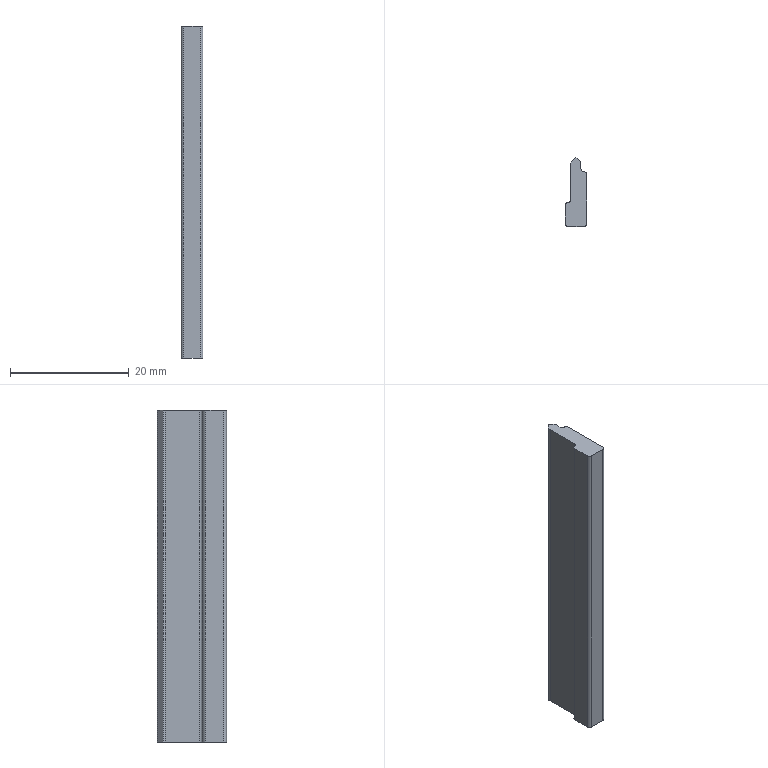Part | NX | features BREP 2 | 2 solids | 34 faces | box 3.7 x 11.653 x 56 mm | volume 3605 mm3 | plane 18 | cylinder 16 | commonest cylinder face diameters 1 x16
STEP:
#1=CARTESIAN_POINT('',(0.6935,5.13,-4.));
#2=VERTEX_POINT('',#1);
#3=CARTESIAN_POINT('',(0.6935,5.13,52.));
#4=VERTEX_POINT('',#3);
#5=CARTESIAN_POINT('',(0.6935,5.13,0.));
#6=DIRECTION('',(0.,0.,1.));
#7=VECTOR('',#6,1000.);
#8=LINE('',#5,#7);
#9=EDGE_CURVE('',#2,#4,#8,.T.);
#10=ORIENTED_EDGE('',*,*,#9,.T.);
#11=CARTESIAN_POINT('',(0.8399,4.776,52.));
#12=VERTEX_POINT('',#11);
#13=CARTESIAN_POINT('',(0.3399,4.776,52.));
#14=DIRECTION('',(0.,0.,1.));
#15=DIRECTION('',(1.,0.,0.));
#16=AXIS2_PLACEMENT_3D('',#13,#14,#15);
#17=CIRCLE('',#16,0.5);
#18=EDGE_CURVE('',#12,#4,#17,.T.);
#19=ORIENTED_EDGE('',*,*,#18,.F.);
#20=CARTESIAN_POINT('',(0.8399,4.776,-4.));
#21=VERTEX_POINT('',#20);
#22=CARTESIAN_POINT('',(0.8399,4.776,0.));
#23=DIRECTION('',(0.,0.,1.));
#24=VECTOR('',#23,1000.);
#25=LINE('',#22,#24);
#26=EDGE_CURVE('',#21,#12,#25,.T.);
#27=ORIENTED_EDGE('',*,*,#26,.F.);
#28=CARTESIAN_POINT('',(0.3399,4.776,-4.));
#29=DIRECTION('',(0.,0.,1.));
#30=DIRECTION('',(1.,0.,0.));
#31=AXIS2_PLACEMENT_3D('',#28,#29,#30);
#32=CIRCLE('',#31,0.5);
#33=EDGE_CURVE('',#21,#2,#32,.T.);
#34=ORIENTED_EDGE('',*,*,#33,.T.);
#35=EDGE_LOOP('',(#10,#19,#27,#34));
#36=FACE_BOUND('',#35,.T.);
#37=CARTESIAN_POINT('',(0.3399,4.776,0.));
#38=DIRECTION('',(0.,0.,1.));
#39=DIRECTION('',(-1.,0.,0.));
#40=AXIS2_PLACEMENT_3D('',#37,#38,#39);
#41=CYLINDRICAL_SURFACE('',#40,0.5);
#42=ADVANCED_FACE('',(#36),#41,.T.);
#43=ORIENTED_EDGE('',*,*,#26,.T.);
#44=CARTESIAN_POINT('',(0.8399,3.873,52.));
#45=VERTEX_POINT('',#44);
#46=CARTESIAN_POINT('',(0.8399,-7.849,52.));
#47=DIRECTION('',(0.,1.,0.));
#48=VECTOR('',#47,1000.);
#49=LINE('',#46,#48);
#50=EDGE_CURVE('',#45,#12,#49,.T.);
#51=ORIENTED_EDGE('',*,*,#50,.F.);
#52=CARTESIAN_POINT('',(0.8399,3.873,-4.));
#53=VERTEX_POINT('',#52);
#54=CARTESIAN_POINT('',(0.8399,3.873,0.));
#55=DIRECTION('',(0.,0.,1.));
#56=VECTOR('',#55,1000.);
#57=LINE('',#54,#56);
#58=EDGE_CURVE('',#53,#45,#57,.T.);
#59=ORIENTED_EDGE('',*,*,#58,.F.);
#60=CARTESIAN_POINT('',(0.8399,-7.849,-4.));
#61=DIRECTION('',(0.,1.,0.));
#62=VECTOR('',#61,1000.);
#63=LINE('',#60,#62);
#64=EDGE_CURVE('',#53,#21,#63,.T.);
#65=ORIENTED_EDGE('',*,*,#64,.T.);
#66=EDGE_LOOP('',(#43,#51,#59,#65));
#67=FACE_BOUND('',#66,.T.);
#68=CARTESIAN_POINT('',(0.8399,4.776,0.));
#69=DIRECTION('',(-1.,0.,0.));
#70=DIRECTION('',(0.,1.,0.));
#71=AXIS2_PLACEMENT_3D('',#68,#69,#70);
#72=PLANE('',#71);
#73=ADVANCED_FACE('',(#67),#72,.F.);
#74=ORIENTED_EDGE('',*,*,#58,.T.);
#75=CARTESIAN_POINT('',(1.35,3.373,52.));
#76=VERTEX_POINT('',#75);
#77=CARTESIAN_POINT('',(1.34,3.873,52.));
#78=DIRECTION('',(0.,0.,-1.));
#79=DIRECTION('',(1.,0.,0.));
#80=AXIS2_PLACEMENT_3D('',#77,#78,#79);
#81=CIRCLE('',#80,0.5);
#82=EDGE_CURVE('',#76,#45,#81,.T.);
#83=ORIENTED_EDGE('',*,*,#82,.F.);
#84=CARTESIAN_POINT('',(1.35,3.373,-4.));
#85=VERTEX_POINT('',#84);
#86=CARTESIAN_POINT('',(1.35,3.373,52.));
#87=CARTESIAN_POINT('',(1.35,3.373,33.333));
#88=CARTESIAN_POINT('',(1.35,3.373,14.667));
#89=CARTESIAN_POINT('',(1.35,3.373,-4.));
#90=B_SPLINE_CURVE_WITH_KNOTS('',3,(#86,#87,#88,#89),.UNSPECIFIED.,.F.,.F.,(4,4),(0.,1.),.UNSPECIFIED.);
#91=EDGE_CURVE('',#85,#76,#90,.F.);
#92=ORIENTED_EDGE('',*,*,#91,.F.);
#93=CARTESIAN_POINT('',(1.34,3.873,-4.));
#94=DIRECTION('',(0.,0.,-1.));
#95=DIRECTION('',(1.,0.,0.));
#96=AXIS2_PLACEMENT_3D('',#93,#94,#95);
#97=CIRCLE('',#96,0.5);
#98=EDGE_CURVE('',#85,#53,#97,.T.);
#99=ORIENTED_EDGE('',*,*,#98,.T.);
#100=EDGE_LOOP('',(#74,#83,#92,#99));
#101=FACE_BOUND('',#100,.T.);
#102=CARTESIAN_POINT('',(1.34,3.873,0.));
#103=DIRECTION('',(0.,0.,1.));
#104=DIRECTION('',(-1.,0.,0.));
#105=AXIS2_PLACEMENT_3D('',#102,#103,#104);
#106=CYLINDRICAL_SURFACE('',#105,0.5);
#107=ADVANCED_FACE('',(#101),#106,.F.);
#108=ORIENTED_EDGE('',*,*,#91,.T.);
#109=CARTESIAN_POINT('',(1.85,2.873,52.));
#110=VERTEX_POINT('',#109);
#111=CARTESIAN_POINT('',(1.35,2.873,52.));
#112=DIRECTION('',(0.,0.,1.));
#113=DIRECTION('',(1.,0.,0.));
#114=AXIS2_PLACEMENT_3D('',#111,#112,#113);
#115=CIRCLE('',#114,0.5);
#116=EDGE_CURVE('',#110,#76,#115,.T.);
#117=ORIENTED_EDGE('',*,*,#116,.F.);
#118=CARTESIAN_POINT('',(1.85,2.873,-4.));
#119=VERTEX_POINT('',#118);
#120=CARTESIAN_POINT('',(1.85,2.873,0.));
#121=DIRECTION('',(0.,0.,1.));
#122=VECTOR('',#121,1000.);
#123=LINE('',#120,#122);
#124=EDGE_CURVE('',#119,#110,#123,.T.);
#125=ORIENTED_EDGE('',*,*,#124,.F.);
#126=CARTESIAN_POINT('',(1.35,2.873,-4.));
#127=DIRECTION('',(0.,0.,1.));
#128=DIRECTION('',(1.,0.,0.));
#129=AXIS2_PLACEMENT_3D('',#126,#127,#128);
#130=CIRCLE('',#129,0.5);
#131=EDGE_CURVE('',#119,#85,#130,.T.);
#132=ORIENTED_EDGE('',*,*,#131,.T.);
#133=EDGE_LOOP('',(#108,#117,#125,#132));
#134=FACE_BOUND('',#133,.T.);
#135=CARTESIAN_POINT('',(1.35,2.873,0.));
#136=DIRECTION('',(0.,0.,1.));
#137=DIRECTION('',(-1.,0.,0.));
#138=AXIS2_PLACEMENT_3D('',#135,#136,#137);
#139=CYLINDRICAL_SURFACE('',#138,0.5);
#140=ADVANCED_FACE('',(#134),#139,.T.);
#141=ORIENTED_EDGE('',*,*,#124,.T.);
#142=CARTESIAN_POINT('',(1.85,-5.327,52.));
#143=VERTEX_POINT('',#142);
#144=CARTESIAN_POINT('',(1.85,-7.849,52.));
#145=DIRECTION('',(0.,1.,0.));
#146=VECTOR('',#145,1000.);
#147=LINE('',#144,#146);
#148=EDGE_CURVE('',#143,#110,#147,.T.);
#149=ORIENTED_EDGE('',*,*,#148,.F.);
#150=CARTESIAN_POINT('',(1.85,-5.327,-4.));
#151=VERTEX_POINT('',#150);
#152=CARTESIAN_POINT('',(1.85,-5.327,0.));
#153=DIRECTION('',(0.,0.,1.));
#154=VECTOR('',#153,1000.);
#155=LINE('',#152,#154);
#156=EDGE_CURVE('',#151,#143,#155,.T.);
#157=ORIENTED_EDGE('',*,*,#156,.F.);
#158=CARTESIAN_POINT('',(1.85,-7.849,-4.));
#159=DIRECTION('',(0.,1.,0.));
#160=VECTOR('',#159,1000.);
#161=LINE('',#158,#160);
#162=EDGE_CURVE('',#151,#119,#161,.T.);
#163=ORIENTED_EDGE('',*,*,#162,.T.);
#164=EDGE_LOOP('',(#141,#149,#157,#163));
#165=FACE_BOUND('',#164,.T.);
#166=CARTESIAN_POINT('',(1.85,2.873,0.));
#167=DIRECTION('',(-1.,0.,0.));
#168=DIRECTION('',(0.,1.,0.));
#169=AXIS2_PLACEMENT_3D('',#166,#167,#168);
#170=PLANE('',#169);
#171=ADVANCED_FACE('',(#165),#170,.F.);
#172=ORIENTED_EDGE('',*,*,#156,.T.);
#173=CARTESIAN_POINT('',(1.35,-5.827,52.));
#174=VERTEX_POINT('',#173);
#175=CARTESIAN_POINT('',(1.35,-5.327,52.));
#176=DIRECTION('',(0.,0.,1.));
#177=DIRECTION('',(1.,0.,0.));
#178=AXIS2_PLACEMENT_3D('',#175,#176,#177);
#179=CIRCLE('',#178,0.5);
#180=EDGE_CURVE('',#174,#143,#179,.T.);
#181=ORIENTED_EDGE('',*,*,#180,.F.);
#182=CARTESIAN_POINT('',(1.35,-5.827,-4.));
#183=VERTEX_POINT('',#182);
#184=CARTESIAN_POINT('',(1.35,-5.827,0.));
#185=DIRECTION('',(0.,0.,1.));
#186=VECTOR('',#185,1000.);
#187=LINE('',#184,#186);
#188=EDGE_CURVE('',#183,#174,#187,.T.);
#189=ORIENTED_EDGE('',*,*,#188,.F.);
#190=CARTESIAN_POINT('',(1.35,-5.327,-4.));
#191=DIRECTION('',(0.,0.,1.));
#192=DIRECTION('',(1.,0.,0.));
#193=AXIS2_PLACEMENT_3D('',#190,#191,#192);
#194=CIRCLE('',#193,0.5);
#195=EDGE_CURVE('',#183,#151,#194,.T.);
#196=ORIENTED_EDGE('',*,*,#195,.T.);
#197=EDGE_LOOP('',(#172,#181,#189,#196));
#198=FACE_BOUND('',#197,.T.);
#199=CARTESIAN_POINT('',(1.35,-5.327,0.));
#200=DIRECTION('',(0.,0.,1.));
#201=DIRECTION('',(-1.,0.,0.));
#202=AXIS2_PLACEMENT_3D('',#199,#200,#201);
#203=CYLINDRICAL_SURFACE('',#202,0.5);
#204=ADVANCED_FACE('',(#198),#203,.T.);
#205=ORIENTED_EDGE('',*,*,#188,.T.);
#206=CARTESIAN_POINT('',(-1.35,-5.827,52.));
#207=VERTEX_POINT('',#206);
#208=CARTESIAN_POINT('',(12.323,-5.827,52.));
#209=DIRECTION('',(1.,0.,0.));
#210=VECTOR('',#209,1000.);
#211=LINE('',#208,#210);
#212=EDGE_CURVE('',#207,#174,#211,.T.);
#213=ORIENTED_EDGE('',*,*,#212,.F.);
#214=CARTESIAN_POINT('',(-1.35,-5.827,-4.));
#215=VERTEX_POINT('',#214);
#216=CARTESIAN_POINT('',(-1.35,-5.827,0.));
#217=DIRECTION('',(0.,0.,1.));
#218=VECTOR('',#217,1000.);
#219=LINE('',#216,#218);
#220=EDGE_CURVE('',#215,#207,#219,.T.);
#221=ORIENTED_EDGE('',*,*,#220,.F.);
#222=CARTESIAN_POINT('',(12.323,-5.827,-4.));
#223=DIRECTION('',(1.,0.,0.));
#224=VECTOR('',#223,1000.);
#225=LINE('',#222,#224);
#226=EDGE_CURVE('',#215,#183,#225,.T.);
#227=ORIENTED_EDGE('',*,*,#226,.T.);
#228=EDGE_LOOP('',(#205,#213,#221,#227));
#229=FACE_BOUND('',#228,.T.);
#230=CARTESIAN_POINT('',(1.35,-5.827,0.));
#231=DIRECTION('',(0.,1.,0.));
#232=DIRECTION('',(1.,0.,0.));
#233=AXIS2_PLACEMENT_3D('',#230,#231,#232);
#234=PLANE('',#233);
#235=ADVANCED_FACE('',(#229),#234,.F.);
#236=ORIENTED_EDGE('',*,*,#220,.T.);
#237=CARTESIAN_POINT('',(-1.85,-5.327,52.));
#238=VERTEX_POINT('',#237);
#239=CARTESIAN_POINT('',(-1.35,-5.327,52.));
#240=DIRECTION('',(0.,0.,1.));
#241=DIRECTION('',(1.,0.,0.));
#242=AXIS2_PLACEMENT_3D('',#239,#240,#241);
#243=CIRCLE('',#242,0.5);
#244=EDGE_CURVE('',#238,#207,#243,.T.);
#245=ORIENTED_EDGE('',*,*,#244,.F.);
#246=CARTESIAN_POINT('',(-1.85,-5.327,-4.));
#247=VERTEX_POINT('',#246);
#248=CARTESIAN_POINT('',(-1.85,-5.327,0.));
#249=DIRECTION('',(0.,0.,1.));
#250=VECTOR('',#249,1000.);
#251=LINE('',#248,#250);
#252=EDGE_CURVE('',#247,#238,#251,.T.);
#253=ORIENTED_EDGE('',*,*,#252,.F.);
#254=CARTESIAN_POINT('',(-1.35,-5.327,-4.));
#255=DIRECTION('',(0.,0.,1.));
#256=DIRECTION('',(1.,0.,0.));
#257=AXIS2_PLACEMENT_3D('',#254,#255,#256);
#258=CIRCLE('',#257,0.5);
#259=EDGE_CURVE('',#247,#215,#258,.T.);
#260=ORIENTED_EDGE('',*,*,#259,.T.);
#261=EDGE_LOOP('',(#236,#245,#253,#260));
#262=FACE_BOUND('',#261,.T.);
#263=CARTESIAN_POINT('',(-1.35,-5.327,0.));
#264=DIRECTION('',(0.,0.,1.));
#265=DIRECTION('',(-1.,0.,0.));
#266=AXIS2_PLACEMENT_3D('',#263,#264,#265);
#267=CYLINDRICAL_SURFACE('',#266,0.5);
#268=ADVANCED_FACE('',(#262),#267,.T.);
#269=ORIENTED_EDGE('',*,*,#252,.T.);
#270=CARTESIAN_POINT('',(-1.85,-2.327,52.));
#271=VERTEX_POINT('',#270);
#272=CARTESIAN_POINT('',(-1.85,-7.849,52.));
#273=DIRECTION('',(0.,-1.,0.));
#274=VECTOR('',#273,1000.);
#275=LINE('',#272,#274);
#276=EDGE_CURVE('',#271,#238,#275,.T.);
#277=ORIENTED_EDGE('',*,*,#276,.F.);
#278=CARTESIAN_POINT('',(-1.85,-2.327,-4.));
#279=VERTEX_POINT('',#278);
#280=CARTESIAN_POINT('',(-1.85,-2.327,0.));
#281=DIRECTION('',(0.,0.,1.));
#282=VECTOR('',#281,1000.);
#283=LINE('',#280,#282);
#284=EDGE_CURVE('',#279,#271,#283,.T.);
#285=ORIENTED_EDGE('',*,*,#284,.F.);
#286=CARTESIAN_POINT('',(-1.85,-7.849,-4.));
#287=DIRECTION('',(0.,-1.,0.));
#288=VECTOR('',#287,1000.);
#289=LINE('',#286,#288);
#290=EDGE_CURVE('',#279,#247,#289,.T.);
#291=ORIENTED_EDGE('',*,*,#290,.T.);
#292=EDGE_LOOP('',(#269,#277,#285,#291));
#293=FACE_BOUND('',#292,.T.);
#294=CARTESIAN_POINT('',(-1.85,-5.327,0.));
#295=DIRECTION('',(1.,0.,0.));
#296=DIRECTION('',(0.,-1.,0.));
#297=AXIS2_PLACEMENT_3D('',#294,#295,#296);
#298=PLANE('',#297);
#299=ADVANCED_FACE('',(#293),#298,.F.);
#300=ORIENTED_EDGE('',*,*,#284,.T.);
#301=CARTESIAN_POINT('',(-1.35,-1.827,52.));
#302=VERTEX_POINT('',#301);
#303=CARTESIAN_POINT('',(-1.35,-2.327,52.));
#304=DIRECTION('',(0.,0.,1.));
#305=DIRECTION('',(1.,0.,0.));
#306=AXIS2_PLACEMENT_3D('',#303,#304,#305);
#307=CIRCLE('',#306,0.5);
#308=EDGE_CURVE('',#302,#271,#307,.T.);
#309=ORIENTED_EDGE('',*,*,#308,.F.);
#310=CARTESIAN_POINT('',(-1.35,-1.827,-4.));
#311=VERTEX_POINT('',#310);
#312=CARTESIAN_POINT('',(-1.35,-1.827,0.));
#313=DIRECTION('',(0.,0.,1.));
#314=VECTOR('',#313,1000.);
#315=LINE('',#312,#314);
#316=EDGE_CURVE('',#311,#302,#315,.T.);
#317=ORIENTED_EDGE('',*,*,#316,.F.);
#318=CARTESIAN_POINT('',(-1.35,-2.327,-4.));
#319=DIRECTION('',(0.,0.,1.));
#320=DIRECTION('',(1.,0.,0.));
#321=AXIS2_PLACEMENT_3D('',#318,#319,#320);
#322=CIRCLE('',#321,0.5);
#323=EDGE_CURVE('',#311,#279,#322,.T.);
#324=ORIENTED_EDGE('',*,*,#323,.T.);
#325=EDGE_LOOP('',(#300,#309,#317,#324));
#326=FACE_BOUND('',#325,.T.);
#327=CARTESIAN_POINT('',(-1.35,-2.327,0.));
#328=DIRECTION('',(0.,0.,1.));
#329=DIRECTION('',(-1.,0.,0.));
#330=AXIS2_PLACEMENT_3D('',#327,#328,#329);
#331=CYLINDRICAL_SURFACE('',#330,0.5);
#332=ADVANCED_FACE('',(#326),#331,.T.);
#333=ORIENTED_EDGE('',*,*,#316,.T.);
#334=CARTESIAN_POINT('',(-0.85,-1.327,52.));
#335=VERTEX_POINT('',#334);
#336=CARTESIAN_POINT('',(-1.35,-1.327,52.));
#337=DIRECTION('',(0.,0.,-1.));
#338=DIRECTION('',(1.,0.,0.));
#339=AXIS2_PLACEMENT_3D('',#336,#337,#338);
#340=CIRCLE('',#339,0.5);
#341=EDGE_CURVE('',#335,#302,#340,.T.);
#342=ORIENTED_EDGE('',*,*,#341,.F.);
#343=CARTESIAN_POINT('',(-0.85,-1.327,-4.));
#344=VERTEX_POINT('',#343);
#345=CARTESIAN_POINT('',(-0.85,-1.327,0.));
#346=DIRECTION('',(0.,0.,1.));
#347=VECTOR('',#346,1000.);
#348=LINE('',#345,#347);
#349=EDGE_CURVE('',#344,#335,#348,.T.);
#350=ORIENTED_EDGE('',*,*,#349,.F.);
#351=CARTESIAN_POINT('',(-1.35,-1.327,-4.));
#352=DIRECTION('',(0.,0.,-1.));
#353=DIRECTION('',(1.,0.,0.));
#354=AXIS2_PLACEMENT_3D('',#351,#352,#353);
#355=CIRCLE('',#354,0.5);
#356=EDGE_CURVE('',#344,#311,#355,.T.);
#357=ORIENTED_EDGE('',*,*,#356,.T.);
#358=EDGE_LOOP('',(#333,#342,#350,#357));
#359=FACE_BOUND('',#358,.T.);
#360=CARTESIAN_POINT('',(-1.35,-1.327,0.));
#361=DIRECTION('',(0.,0.,1.));
#362=DIRECTION('',(-1.,0.,0.));
#363=AXIS2_PLACEMENT_3D('',#360,#361,#362);
#364=CYLINDRICAL_SURFACE('',#363,0.5);
#365=ADVANCED_FACE('',(#359),#364,.F.);
#366=ORIENTED_EDGE('',*,*,#349,.T.);
#367=CARTESIAN_POINT('',(-0.85,4.473,52.));
#368=VERTEX_POINT('',#367);
#369=CARTESIAN_POINT('',(-0.85,-7.849,52.));
#370=DIRECTION('',(0.,-1.,0.));
#371=VECTOR('',#370,1000.);
#372=LINE('',#369,#371);
#373=EDGE_CURVE('',#368,#335,#372,.T.);
#374=ORIENTED_EDGE('',*,*,#373,.F.);
#375=CARTESIAN_POINT('',(-0.85,4.473,-4.));
#376=VERTEX_POINT('',#375);
#377=CARTESIAN_POINT('',(-0.85,4.473,0.));
#378=DIRECTION('',(0.,0.,1.));
#379=VECTOR('',#378,1000.);
#380=LINE('',#377,#379);
#381=EDGE_CURVE('',#376,#368,#380,.T.);
#382=ORIENTED_EDGE('',*,*,#381,.F.);
#383=CARTESIAN_POINT('',(-0.85,-7.849,-4.));
#384=DIRECTION('',(0.,-1.,0.));
#385=VECTOR('',#384,1000.);
#386=LINE('',#383,#385);
#387=EDGE_CURVE('',#376,#344,#386,.T.);
#388=ORIENTED_EDGE('',*,*,#387,.T.);
#389=EDGE_LOOP('',(#366,#374,#382,#388));
#390=FACE_BOUND('',#389,.T.);
#391=CARTESIAN_POINT('',(-0.85,-1.327,0.));
#392=DIRECTION('',(1.,0.,0.));
#393=DIRECTION('',(0.,-1.,0.));
#394=AXIS2_PLACEMENT_3D('',#391,#392,#393);
#395=PLANE('',#394);
#396=ADVANCED_FACE('',(#390),#395,.F.);
#397=ORIENTED_EDGE('',*,*,#381,.T.);
#398=CARTESIAN_POINT('',(-0.9972,4.828,52.));
#399=VERTEX_POINT('',#398);
#400=CARTESIAN_POINT('',(-1.35,4.473,52.));
#401=DIRECTION('',(0.,0.,-1.));
#402=DIRECTION('',(1.,0.,0.));
#403=AXIS2_PLACEMENT_3D('',#400,#401,#402);
#404=CIRCLE('',#403,0.5);
#405=EDGE_CURVE('',#399,#368,#404,.T.);
#406=ORIENTED_EDGE('',*,*,#405,.F.);
#407=CARTESIAN_POINT('',(-0.9972,4.828,-4.));
#408=VERTEX_POINT('',#407);
#409=CARTESIAN_POINT('',(-0.9972,4.828,0.));
#410=DIRECTION('',(0.,0.,1.));
#411=VECTOR('',#410,1000.);
#412=LINE('',#409,#411);
#413=EDGE_CURVE('',#408,#399,#412,.T.);
#414=ORIENTED_EDGE('',*,*,#413,.F.);
#415=CARTESIAN_POINT('',(-1.35,4.473,-4.));
#416=DIRECTION('',(0.,0.,-1.));
#417=DIRECTION('',(1.,0.,0.));
#418=AXIS2_PLACEMENT_3D('',#415,#416,#417);
#419=CIRCLE('',#418,0.5);
#420=EDGE_CURVE('',#408,#376,#419,.T.);
#421=ORIENTED_EDGE('',*,*,#420,.T.);
#422=EDGE_LOOP('',(#397,#406,#414,#421));
#423=FACE_BOUND('',#422,.T.);
#424=CARTESIAN_POINT('',(-1.35,4.473,0.));
#425=DIRECTION('',(0.,0.,1.));
#426=DIRECTION('',(-1.,0.,0.));
#427=AXIS2_PLACEMENT_3D('',#424,#425,#426);
#428=CYLINDRICAL_SURFACE('',#427,0.5);
#429=ADVANCED_FACE('',(#423),#428,.F.);
#430=ORIENTED_EDGE('',*,*,#413,.T.);
#431=CARTESIAN_POINT('',(-0.002816,5.826,52.));
#432=VERTEX_POINT('',#431);
#433=CARTESIAN_POINT('',(-0.7029,5.123,52.));
#434=DIRECTION('',(-0.7056,-0.7086,0.));
#435=VECTOR('',#434,1000.);
#436=LINE('',#433,#435);
#437=EDGE_CURVE('',#432,#399,#436,.T.);
#438=ORIENTED_EDGE('',*,*,#437,.F.);
#439=CARTESIAN_POINT('',(-0.002816,5.826,-4.));
#440=VERTEX_POINT('',#439);
#441=CARTESIAN_POINT('',(-0.002816,5.826,0.));
#442=DIRECTION('',(0.,0.,1.));
#443=VECTOR('',#442,1000.);
#444=LINE('',#441,#443);
#445=EDGE_CURVE('',#440,#432,#444,.T.);
#446=ORIENTED_EDGE('',*,*,#445,.F.);
#447=CARTESIAN_POINT('',(-0.7029,5.123,-4.));
#448=DIRECTION('',(-0.7056,-0.7086,0.));
#449=VECTOR('',#448,1000.);
#450=LINE('',#447,#449);
#451=EDGE_CURVE('',#440,#408,#450,.T.);
#452=ORIENTED_EDGE('',*,*,#451,.T.);
#453=EDGE_LOOP('',(#430,#438,#446,#452));
#454=FACE_BOUND('',#453,.T.);
#455=CARTESIAN_POINT('',(-0.7029,5.123,0.));
#456=DIRECTION('',(0.7086,-0.7056,0.));
#457=DIRECTION('',(-0.7056,-0.7086,0.));
#458=AXIS2_PLACEMENT_3D('',#455,#456,#457);
#459=PLANE('',#458);
#460=ADVANCED_FACE('',(#454),#459,.F.);
#461=CARTESIAN_POINT('',(-0.003553,5.827,-4.));
#462=DIRECTION('',(-0.7071,0.7071,0.));
#463=VECTOR('',#462,1000.);
#464=LINE('',#461,#463);
#465=EDGE_CURVE('',#2,#440,#464,.T.);
#466=ORIENTED_EDGE('',*,*,#465,.T.);
#467=ORIENTED_EDGE('',*,*,#445,.T.);
#468=CARTESIAN_POINT('',(-0.003553,5.827,52.));
#469=DIRECTION('',(-0.7071,0.7071,0.));
#470=VECTOR('',#469,1000.);
#471=LINE('',#468,#470);
#472=EDGE_CURVE('',#4,#432,#471,.T.);
#473=ORIENTED_EDGE('',*,*,#472,.F.);
#474=ORIENTED_EDGE('',*,*,#9,.F.);
#475=EDGE_LOOP('',(#466,#467,#473,#474));
#476=FACE_BOUND('',#475,.T.);
#477=CARTESIAN_POINT('',(-0.003553,5.827,0.));
#478=DIRECTION('',(-0.7071,-0.7071,0.));
#479=DIRECTION('',(-0.7071,0.7071,0.));
#480=AXIS2_PLACEMENT_3D('',#477,#478,#479);
#481=PLANE('',#480);
#482=ADVANCED_FACE('',(#476),#481,.F.);
#483=ORIENTED_EDGE('',*,*,#437,.T.);
#484=ORIENTED_EDGE('',*,*,#405,.T.);
#485=ORIENTED_EDGE('',*,*,#373,.T.);
#486=ORIENTED_EDGE('',*,*,#341,.T.);
#487=ORIENTED_EDGE('',*,*,#308,.T.);
#488=ORIENTED_EDGE('',*,*,#276,.T.);
#489=ORIENTED_EDGE('',*,*,#244,.T.);
#490=ORIENTED_EDGE('',*,*,#212,.T.);
#491=ORIENTED_EDGE('',*,*,#180,.T.);
#492=ORIENTED_EDGE('',*,*,#148,.T.);
#493=ORIENTED_EDGE('',*,*,#116,.T.);
#494=ORIENTED_EDGE('',*,*,#82,.T.);
#495=ORIENTED_EDGE('',*,*,#50,.T.);
#496=ORIENTED_EDGE('',*,*,#18,.T.);
#497=ORIENTED_EDGE('',*,*,#472,.T.);
#498=EDGE_LOOP('',(#483,#484,#485,#486,#487,#488,#489,#490,#491,#492,#493,#494,#495,#496,#497));
#499=FACE_BOUND('',#498,.T.);
#500=CARTESIAN_POINT('',(12.323,-7.849,52.));
#501=DIRECTION('',(0.,0.,1.));
#502=DIRECTION('',(-1.,0.,0.));
#503=AXIS2_PLACEMENT_3D('',#500,#501,#502);
#504=PLANE('',#503);
#505=ADVANCED_FACE('',(#499),#504,.T.);
#506=ORIENTED_EDGE('',*,*,#451,.F.);
#507=ORIENTED_EDGE('',*,*,#465,.F.);
#508=ORIENTED_EDGE('',*,*,#33,.F.);
#509=ORIENTED_EDGE('',*,*,#64,.F.);
#510=ORIENTED_EDGE('',*,*,#98,.F.);
#511=ORIENTED_EDGE('',*,*,#131,.F.);
#512=ORIENTED_EDGE('',*,*,#162,.F.);
#513=ORIENTED_EDGE('',*,*,#195,.F.);
#514=ORIENTED_EDGE('',*,*,#226,.F.);
#515=ORIENTED_EDGE('',*,*,#259,.F.);
#516=ORIENTED_EDGE('',*,*,#290,.F.);
#517=ORIENTED_EDGE('',*,*,#323,.F.);
#518=ORIENTED_EDGE('',*,*,#356,.F.);
#519=ORIENTED_EDGE('',*,*,#387,.F.);
#520=ORIENTED_EDGE('',*,*,#420,.F.);
#521=EDGE_LOOP('',(#506,#507,#508,#509,#510,#511,#512,#513,#514,#515,#516,#517,#518,#519,#520));
#522=FACE_BOUND('',#521,.T.);
#523=CARTESIAN_POINT('',(12.323,-7.849,-4.));
#524=DIRECTION('',(0.,0.,1.));
#525=DIRECTION('',(-1.,0.,0.));
#526=AXIS2_PLACEMENT_3D('',#523,#524,#525);
#527=PLANE('',#526);
#528=ADVANCED_FACE('',(#522),#527,.F.);
#529=CLOSED_SHELL('',(#42,#73,#107,#140,#171,#204,#235,#268,#299,#332,#365,#396,#429,#460,#482,#505,#528));
#530=MANIFOLD_SOLID_BREP('',#529);
#531=CARTESIAN_POINT('',(0.6935,5.13,-4.));
#532=VERTEX_POINT('',#531);
#533=CARTESIAN_POINT('',(0.6935,5.13,52.));
#534=VERTEX_POINT('',#533);
#535=CARTESIAN_POINT('',(0.6935,5.13,0.));
#536=DIRECTION('',(0.,0.,1.));
#537=VECTOR('',#536,1000.);
#538=LINE('',#535,#537);
#539=EDGE_CURVE('',#532,#534,#538,.T.);
#540=ORIENTED_EDGE('',*,*,#539,.T.);
#541=CARTESIAN_POINT('',(0.8399,4.776,52.));
#542=VERTEX_POINT('',#541);
#543=CARTESIAN_POINT('',(0.3399,4.776,52.));
#544=DIRECTION('',(0.,0.,1.));
#545=DIRECTION('',(1.,0.,0.));
#546=AXIS2_PLACEMENT_3D('',#543,#544,#545);
#547=CIRCLE('',#546,0.5);
#548=EDGE_CURVE('',#542,#534,#547,.T.);
#549=ORIENTED_EDGE('',*,*,#548,.F.);
#550=CARTESIAN_POINT('',(0.8399,4.776,-4.));
#551=VERTEX_POINT('',#550);
#552=CARTESIAN_POINT('',(0.8399,4.776,0.));
#553=DIRECTION('',(0.,0.,1.));
#554=VECTOR('',#553,1000.);
#555=LINE('',#552,#554);
#556=EDGE_CURVE('',#551,#542,#555,.T.);
#557=ORIENTED_EDGE('',*,*,#556,.F.);
#558=CARTESIAN_POINT('',(0.3399,4.776,-4.));
#559=DIRECTION('',(0.,0.,1.));
#560=DIRECTION('',(1.,0.,0.));
#561=AXIS2_PLACEMENT_3D('',#558,#559,#560);
#562=CIRCLE('',#561,0.5);
#563=EDGE_CURVE('',#551,#532,#562,.T.);
#564=ORIENTED_EDGE('',*,*,#563,.T.);
#565=EDGE_LOOP('',(#540,#549,#557,#564));
#566=FACE_BOUND('',#565,.T.);
#567=CARTESIAN_POINT('',(0.3399,4.776,0.));
#568=DIRECTION('',(0.,0.,1.));
#569=DIRECTION('',(-1.,0.,0.));
#570=AXIS2_PLACEMENT_3D('',#567,#568,#569);
#571=CYLINDRICAL_SURFACE('',#570,0.5);
#572=ADVANCED_FACE('',(#566),#571,.T.);
#573=ORIENTED_EDGE('',*,*,#556,.T.);
#574=CARTESIAN_POINT('',(0.8399,3.873,52.));
#575=VERTEX_POINT('',#574);
#576=CARTESIAN_POINT('',(0.8399,-7.849,52.));
#577=DIRECTION('',(0.,1.,0.));
#578=VECTOR('',#577,1000.);
#579=LINE('',#576,#578);
#580=EDGE_CURVE('',#575,#542,#579,.T.);
#581=ORIENTED_EDGE('',*,*,#580,.F.);
#582=CARTESIAN_POINT('',(0.8399,3.873,-4.));
#583=VERTEX_POINT('',#582);
#584=CARTESIAN_POINT('',(0.8399,3.873,0.));
#585=DIRECTION('',(0.,0.,1.));
#586=VECTOR('',#585,1000.);
#587=LINE('',#584,#586);
#588=EDGE_CURVE('',#583,#575,#587,.T.);
#589=ORIENTED_EDGE('',*,*,#588,.F.);
#590=CARTESIAN_POINT('',(0.8399,-7.849,-4.));
#591=DIRECTION('',(0.,1.,0.));
#592=VECTOR('',#591,1000.);
#593=LINE('',#590,#592);
#594=EDGE_CURVE('',#583,#551,#593,.T.);
#595=ORIENTED_EDGE('',*,*,#594,.T.);
#596=EDGE_LOOP('',(#573,#581,#589,#595));
#597=FACE_BOUND('',#596,.T.);
#598=CARTESIAN_POINT('',(0.8399,4.776,0.));
#599=DIRECTION('',(-1.,0.,0.));
#600=DIRECTION('',(0.,1.,0.));
#601=AXIS2_PLACEMENT_3D('',#598,#599,#600);
#602=PLANE('',#601);
#603=ADVANCED_FACE('',(#597),#602,.F.);
#604=ORIENTED_EDGE('',*,*,#588,.T.);
#605=CARTESIAN_POINT('',(1.35,3.373,52.));
#606=VERTEX_POINT('',#605);
#607=CARTESIAN_POINT('',(1.34,3.873,52.));
#608=DIRECTION('',(0.,0.,-1.));
#609=DIRECTION('',(1.,0.,0.));
#610=AXIS2_PLACEMENT_3D('',#607,#608,#609);
#611=CIRCLE('',#610,0.5);
#612=EDGE_CURVE('',#606,#575,#611,.T.);
#613=ORIENTED_EDGE('',*,*,#612,.F.);
#614=CARTESIAN_POINT('',(1.35,3.373,-4.));
#615=VERTEX_POINT('',#614);
#616=CARTESIAN_POINT('',(1.35,3.373,52.));
#617=CARTESIAN_POINT('',(1.35,3.373,33.333));
#618=CARTESIAN_POINT('',(1.35,3.373,14.667));
#619=CARTESIAN_POINT('',(1.35,3.373,-4.));
#620=B_SPLINE_CURVE_WITH_KNOTS('',3,(#616,#617,#618,#619),.UNSPECIFIED.,.F.,.F.,(4,4),(0.,1.),.UNSPECIFIED.);
#621=EDGE_CURVE('',#615,#606,#620,.F.);
#622=ORIENTED_EDGE('',*,*,#621,.F.);
#623=CARTESIAN_POINT('',(1.34,3.873,-4.));
#624=DIRECTION('',(0.,0.,-1.));
#625=DIRECTION('',(1.,0.,0.));
#626=AXIS2_PLACEMENT_3D('',#623,#624,#625);
#627=CIRCLE('',#626,0.5);
#628=EDGE_CURVE('',#615,#583,#627,.T.);
#629=ORIENTED_EDGE('',*,*,#628,.T.);
#630=EDGE_LOOP('',(#604,#613,#622,#629));
#631=FACE_BOUND('',#630,.T.);
#632=CARTESIAN_POINT('',(1.34,3.873,0.));
#633=DIRECTION('',(0.,0.,1.));
#634=DIRECTION('',(-1.,0.,0.));
#635=AXIS2_PLACEMENT_3D('',#632,#633,#634);
#636=CYLINDRICAL_SURFACE('',#635,0.5);
#637=ADVANCED_FACE('',(#631),#636,.F.);
#638=ORIENTED_EDGE('',*,*,#621,.T.);
#639=CARTESIAN_POINT('',(1.85,2.873,52.));
#640=VERTEX_POINT('',#639);
#641=CARTESIAN_POINT('',(1.35,2.873,52.));
#642=DIRECTION('',(0.,0.,1.));
#643=DIRECTION('',(1.,0.,0.));
#644=AXIS2_PLACEMENT_3D('',#641,#642,#643);
#645=CIRCLE('',#644,0.5);
#646=EDGE_CURVE('',#640,#606,#645,.T.);
#647=ORIENTED_EDGE('',*,*,#646,.F.);
#648=CARTESIAN_POINT('',(1.85,2.873,-4.));
#649=VERTEX_POINT('',#648);
#650=CARTESIAN_POINT('',(1.85,2.873,0.));
#651=DIRECTION('',(0.,0.,1.));
#652=VECTOR('',#651,1000.);
#653=LINE('',#650,#652);
#654=EDGE_CURVE('',#649,#640,#653,.T.);
#655=ORIENTED_EDGE('',*,*,#654,.F.);
#656=CARTESIAN_POINT('',(1.35,2.873,-4.));
#657=DIRECTION('',(0.,0.,1.));
#658=DIRECTION('',(1.,0.,0.));
#659=AXIS2_PLACEMENT_3D('',#656,#657,#658);
#660=CIRCLE('',#659,0.5);
#661=EDGE_CURVE('',#649,#615,#660,.T.);
#662=ORIENTED_EDGE('',*,*,#661,.T.);
#663=EDGE_LOOP('',(#638,#647,#655,#662));
#664=FACE_BOUND('',#663,.T.);
#665=CARTESIAN_POINT('',(1.35,2.873,0.));
#666=DIRECTION('',(0.,0.,1.));
#667=DIRECTION('',(-1.,0.,0.));
#668=AXIS2_PLACEMENT_3D('',#665,#666,#667);
#669=CYLINDRICAL_SURFACE('',#668,0.5);
#670=ADVANCED_FACE('',(#664),#669,.T.);
#671=ORIENTED_EDGE('',*,*,#654,.T.);
#672=CARTESIAN_POINT('',(1.85,-5.327,52.));
#673=VERTEX_POINT('',#672);
#674=CARTESIAN_POINT('',(1.85,-7.849,52.));
#675=DIRECTION('',(0.,1.,0.));
#676=VECTOR('',#675,1000.);
#677=LINE('',#674,#676);
#678=EDGE_CURVE('',#673,#640,#677,.T.);
#679=ORIENTED_EDGE('',*,*,#678,.F.);
#680=CARTESIAN_POINT('',(1.85,-5.327,-4.));
#681=VERTEX_POINT('',#680);
#682=CARTESIAN_POINT('',(1.85,-5.327,0.));
#683=DIRECTION('',(0.,0.,1.));
#684=VECTOR('',#683,1000.);
#685=LINE('',#682,#684);
#686=EDGE_CURVE('',#681,#673,#685,.T.);
#687=ORIENTED_EDGE('',*,*,#686,.F.);
#688=CARTESIAN_POINT('',(1.85,-7.849,-4.));
#689=DIRECTION('',(0.,1.,0.));
#690=VECTOR('',#689,1000.);
#691=LINE('',#688,#690);
#692=EDGE_CURVE('',#681,#649,#691,.T.);
#693=ORIENTED_EDGE('',*,*,#692,.T.);
#694=EDGE_LOOP('',(#671,#679,#687,#693));
#695=FACE_BOUND('',#694,.T.);
#696=CARTESIAN_POINT('',(1.85,2.873,0.));
#697=DIRECTION('',(-1.,0.,0.));
#698=DIRECTION('',(0.,1.,0.));
#699=AXIS2_PLACEMENT_3D('',#696,#697,#698);
#700=PLANE('',#699);
#701=ADVANCED_FACE('',(#695),#700,.F.);
#702=ORIENTED_EDGE('',*,*,#686,.T.);
#703=CARTESIAN_POINT('',(1.35,-5.827,52.));
#704=VERTEX_POINT('',#703);
#705=CARTESIAN_POINT('',(1.35,-5.327,52.));
#706=DIRECTION('',(0.,0.,1.));
#707=DIRECTION('',(1.,0.,0.));
#708=AXIS2_PLACEMENT_3D('',#705,#706,#707);
#709=CIRCLE('',#708,0.5);
#710=EDGE_CURVE('',#704,#673,#709,.T.);
#711=ORIENTED_EDGE('',*,*,#710,.F.);
#712=CARTESIAN_POINT('',(1.35,-5.827,-4.));
#713=VERTEX_POINT('',#712);
#714=CARTESIAN_POINT('',(1.35,-5.827,0.));
#715=DIRECTION('',(0.,0.,1.));
#716=VECTOR('',#715,1000.);
#717=LINE('',#714,#716);
#718=EDGE_CURVE('',#713,#704,#717,.T.);
#719=ORIENTED_EDGE('',*,*,#718,.F.);
#720=CARTESIAN_POINT('',(1.35,-5.327,-4.));
#721=DIRECTION('',(0.,0.,1.));
#722=DIRECTION('',(1.,0.,0.));
#723=AXIS2_PLACEMENT_3D('',#720,#721,#722);
#724=CIRCLE('',#723,0.5);
#725=EDGE_CURVE('',#713,#681,#724,.T.);
#726=ORIENTED_EDGE('',*,*,#725,.T.);
#727=EDGE_LOOP('',(#702,#711,#719,#726));
#728=FACE_BOUND('',#727,.T.);
#729=CARTESIAN_POINT('',(1.35,-5.327,0.));
#730=DIRECTION('',(0.,0.,1.));
#731=DIRECTION('',(-1.,0.,0.));
#732=AXIS2_PLACEMENT_3D('',#729,#730,#731);
#733=CYLINDRICAL_SURFACE('',#732,0.5);
#734=ADVANCED_FACE('',(#728),#733,.T.);
#735=ORIENTED_EDGE('',*,*,#718,.T.);
#736=CARTESIAN_POINT('',(-1.35,-5.827,52.));
#737=VERTEX_POINT('',#736);
#738=CARTESIAN_POINT('',(12.323,-5.827,52.));
#739=DIRECTION('',(1.,0.,0.));
#740=VECTOR('',#739,1000.);
#741=LINE('',#738,#740);
#742=EDGE_CURVE('',#737,#704,#741,.T.);
#743=ORIENTED_EDGE('',*,*,#742,.F.);
#744=CARTESIAN_POINT('',(-1.35,-5.827,-4.));
#745=VERTEX_POINT('',#744);
#746=CARTESIAN_POINT('',(-1.35,-5.827,0.));
#747=DIRECTION('',(0.,0.,1.));
#748=VECTOR('',#747,1000.);
#749=LINE('',#746,#748);
#750=EDGE_CURVE('',#745,#737,#749,.T.);
#751=ORIENTED_EDGE('',*,*,#750,.F.);
#752=CARTESIAN_POINT('',(12.323,-5.827,-4.));
#753=DIRECTION('',(1.,0.,0.));
#754=VECTOR('',#753,1000.);
#755=LINE('',#752,#754);
#756=EDGE_CURVE('',#745,#713,#755,.T.);
#757=ORIENTED_EDGE('',*,*,#756,.T.);
#758=EDGE_LOOP('',(#735,#743,#751,#757));
#759=FACE_BOUND('',#758,.T.);
#760=CARTESIAN_POINT('',(1.35,-5.827,0.));
#761=DIRECTION('',(0.,1.,0.));
#762=DIRECTION('',(1.,0.,0.));
#763=AXIS2_PLACEMENT_3D('',#760,#761,#762);
#764=PLANE('',#763);
#765=ADVANCED_FACE('',(#759),#764,.F.);
#766=ORIENTED_EDGE('',*,*,#750,.T.);
#767=CARTESIAN_POINT('',(-1.85,-5.327,52.));
#768=VERTEX_POINT('',#767);
#769=CARTESIAN_POINT('',(-1.35,-5.327,52.));
#770=DIRECTION('',(0.,0.,1.));
#771=DIRECTION('',(1.,0.,0.));
#772=AXIS2_PLACEMENT_3D('',#769,#770,#771);
#773=CIRCLE('',#772,0.5);
#774=EDGE_CURVE('',#768,#737,#773,.T.);
#775=ORIENTED_EDGE('',*,*,#774,.F.);
#776=CARTESIAN_POINT('',(-1.85,-5.327,-4.));
#777=VERTEX_POINT('',#776);
#778=CARTESIAN_POINT('',(-1.85,-5.327,0.));
#779=DIRECTION('',(0.,0.,1.));
#780=VECTOR('',#779,1000.);
#781=LINE('',#778,#780);
#782=EDGE_CURVE('',#777,#768,#781,.T.);
#783=ORIENTED_EDGE('',*,*,#782,.F.);
#784=CARTESIAN_POINT('',(-1.35,-5.327,-4.));
#785=DIRECTION('',(0.,0.,1.));
#786=DIRECTION('',(1.,0.,0.));
#787=AXIS2_PLACEMENT_3D('',#784,#785,#786);
#788=CIRCLE('',#787,0.5);
#789=EDGE_CURVE('',#777,#745,#788,.T.);
#790=ORIENTED_EDGE('',*,*,#789,.T.);
#791=EDGE_LOOP('',(#766,#775,#783,#790));
#792=FACE_BOUND('',#791,.T.);
#793=CARTESIAN_POINT('',(-1.35,-5.327,0.));
#794=DIRECTION('',(0.,0.,1.));
#795=DIRECTION('',(-1.,0.,0.));
#796=AXIS2_PLACEMENT_3D('',#793,#794,#795);
#797=CYLINDRICAL_SURFACE('',#796,0.5);
#798=ADVANCED_FACE('',(#792),#797,.T.);
#799=ORIENTED_EDGE('',*,*,#782,.T.);
#800=CARTESIAN_POINT('',(-1.85,-2.327,52.));
#801=VERTEX_POINT('',#800);
#802=CARTESIAN_POINT('',(-1.85,-7.849,52.));
#803=DIRECTION('',(0.,-1.,0.));
#804=VECTOR('',#803,1000.);
#805=LINE('',#802,#804);
#806=EDGE_CURVE('',#801,#768,#805,.T.);
#807=ORIENTED_EDGE('',*,*,#806,.F.);
#808=CARTESIAN_POINT('',(-1.85,-2.327,-4.));
#809=VERTEX_POINT('',#808);
#810=CARTESIAN_POINT('',(-1.85,-2.327,0.));
#811=DIRECTION('',(0.,0.,1.));
#812=VECTOR('',#811,1000.);
#813=LINE('',#810,#812);
#814=EDGE_CURVE('',#809,#801,#813,.T.);
#815=ORIENTED_EDGE('',*,*,#814,.F.);
#816=CARTESIAN_POINT('',(-1.85,-7.849,-4.));
#817=DIRECTION('',(0.,-1.,0.));
#818=VECTOR('',#817,1000.);
#819=LINE('',#816,#818);
#820=EDGE_CURVE('',#809,#777,#819,.T.);
#821=ORIENTED_EDGE('',*,*,#820,.T.);
#822=EDGE_LOOP('',(#799,#807,#815,#821));
#823=FACE_BOUND('',#822,.T.);
#824=CARTESIAN_POINT('',(-1.85,-5.327,0.));
#825=DIRECTION('',(1.,0.,0.));
#826=DIRECTION('',(0.,-1.,0.));
#827=AXIS2_PLACEMENT_3D('',#824,#825,#826);
#828=PLANE('',#827);
#829=ADVANCED_FACE('',(#823),#828,.F.);
#830=ORIENTED_EDGE('',*,*,#814,.T.);
#831=CARTESIAN_POINT('',(-1.35,-1.827,52.));
#832=VERTEX_POINT('',#831);
#833=CARTESIAN_POINT('',(-1.35,-2.327,52.));
#834=DIRECTION('',(0.,0.,1.));
#835=DIRECTION('',(1.,0.,0.));
#836=AXIS2_PLACEMENT_3D('',#833,#834,#835);
#837=CIRCLE('',#836,0.5);
#838=EDGE_CURVE('',#832,#801,#837,.T.);
#839=ORIENTED_EDGE('',*,*,#838,.F.);
#840=CARTESIAN_POINT('',(-1.35,-1.827,-4.));
#841=VERTEX_POINT('',#840);
#842=CARTESIAN_POINT('',(-1.35,-1.827,0.));
#843=DIRECTION('',(0.,0.,1.));
#844=VECTOR('',#843,1000.);
#845=LINE('',#842,#844);
#846=EDGE_CURVE('',#841,#832,#845,.T.);
#847=ORIENTED_EDGE('',*,*,#846,.F.);
#848=CARTESIAN_POINT('',(-1.35,-2.327,-4.));
#849=DIRECTION('',(0.,0.,1.));
#850=DIRECTION('',(1.,0.,0.));
#851=AXIS2_PLACEMENT_3D('',#848,#849,#850);
#852=CIRCLE('',#851,0.5);
#853=EDGE_CURVE('',#841,#809,#852,.T.);
#854=ORIENTED_EDGE('',*,*,#853,.T.);
#855=EDGE_LOOP('',(#830,#839,#847,#854));
#856=FACE_BOUND('',#855,.T.);
#857=CARTESIAN_POINT('',(-1.35,-2.327,0.));
#858=DIRECTION('',(0.,0.,1.));
#859=DIRECTION('',(-1.,0.,0.));
#860=AXIS2_PLACEMENT_3D('',#857,#858,#859);
#861=CYLINDRICAL_SURFACE('',#860,0.5);
#862=ADVANCED_FACE('',(#856),#861,.T.);
#863=ORIENTED_EDGE('',*,*,#846,.T.);
#864=CARTESIAN_POINT('',(-0.85,-1.327,52.));
#865=VERTEX_POINT('',#864);
#866=CARTESIAN_POINT('',(-1.35,-1.327,52.));
#867=DIRECTION('',(0.,0.,-1.));
#868=DIRECTION('',(1.,0.,0.));
#869=AXIS2_PLACEMENT_3D('',#866,#867,#868);
#870=CIRCLE('',#869,0.5);
#871=EDGE_CURVE('',#865,#832,#870,.T.);
#872=ORIENTED_EDGE('',*,*,#871,.F.);
#873=CARTESIAN_POINT('',(-0.85,-1.327,-4.));
#874=VERTEX_POINT('',#873);
#875=CARTESIAN_POINT('',(-0.85,-1.327,0.));
#876=DIRECTION('',(0.,0.,1.));
#877=VECTOR('',#876,1000.);
#878=LINE('',#875,#877);
#879=EDGE_CURVE('',#874,#865,#878,.T.);
#880=ORIENTED_EDGE('',*,*,#879,.F.);
#881=CARTESIAN_POINT('',(-1.35,-1.327,-4.));
#882=DIRECTION('',(0.,0.,-1.));
#883=DIRECTION('',(1.,0.,0.));
#884=AXIS2_PLACEMENT_3D('',#881,#882,#883);
#885=CIRCLE('',#884,0.5);
#886=EDGE_CURVE('',#874,#841,#885,.T.);
#887=ORIENTED_EDGE('',*,*,#886,.T.);
#888=EDGE_LOOP('',(#863,#872,#880,#887));
#889=FACE_BOUND('',#888,.T.);
#890=CARTESIAN_POINT('',(-1.35,-1.327,0.));
#891=DIRECTION('',(0.,0.,1.));
#892=DIRECTION('',(-1.,0.,0.));
#893=AXIS2_PLACEMENT_3D('',#890,#891,#892);
#894=CYLINDRICAL_SURFACE('',#893,0.5);
#895=ADVANCED_FACE('',(#889),#894,.F.);
#896=ORIENTED_EDGE('',*,*,#879,.T.);
#897=CARTESIAN_POINT('',(-0.85,4.473,52.));
#898=VERTEX_POINT('',#897);
#899=CARTESIAN_POINT('',(-0.85,-7.849,52.));
#900=DIRECTION('',(0.,-1.,0.));
#901=VECTOR('',#900,1000.);
#902=LINE('',#899,#901);
#903=EDGE_CURVE('',#898,#865,#902,.T.);
#904=ORIENTED_EDGE('',*,*,#903,.F.);
#905=CARTESIAN_POINT('',(-0.85,4.473,-4.));
#906=VERTEX_POINT('',#905);
#907=CARTESIAN_POINT('',(-0.85,4.473,0.));
#908=DIRECTION('',(0.,0.,1.));
#909=VECTOR('',#908,1000.);
#910=LINE('',#907,#909);
#911=EDGE_CURVE('',#906,#898,#910,.T.);
#912=ORIENTED_EDGE('',*,*,#911,.F.);
#913=CARTESIAN_POINT('',(-0.85,-7.849,-4.));
#914=DIRECTION('',(0.,-1.,0.));
#915=VECTOR('',#914,1000.);
#916=LINE('',#913,#915);
#917=EDGE_CURVE('',#906,#874,#916,.T.);
#918=ORIENTED_EDGE('',*,*,#917,.T.);
#919=EDGE_LOOP('',(#896,#904,#912,#918));
#920=FACE_BOUND('',#919,.T.);
#921=CARTESIAN_POINT('',(-0.85,-1.327,0.));
#922=DIRECTION('',(1.,0.,0.));
#923=DIRECTION('',(0.,-1.,0.));
#924=AXIS2_PLACEMENT_3D('',#921,#922,#923);
#925=PLANE('',#924);
#926=ADVANCED_FACE('',(#920),#925,.F.);
#927=ORIENTED_EDGE('',*,*,#911,.T.);
#928=CARTESIAN_POINT('',(-0.9972,4.828,52.));
#929=VERTEX_POINT('',#928);
#930=CARTESIAN_POINT('',(-1.35,4.473,52.));
#931=DIRECTION('',(0.,0.,-1.));
#932=DIRECTION('',(1.,0.,0.));
#933=AXIS2_PLACEMENT_3D('',#930,#931,#932);
#934=CIRCLE('',#933,0.5);
#935=EDGE_CURVE('',#929,#898,#934,.T.);
#936=ORIENTED_EDGE('',*,*,#935,.F.);
#937=CARTESIAN_POINT('',(-0.9972,4.828,-4.));
#938=VERTEX_POINT('',#937);
#939=CARTESIAN_POINT('',(-0.9972,4.828,0.));
#940=DIRECTION('',(0.,0.,1.));
#941=VECTOR('',#940,1000.);
#942=LINE('',#939,#941);
#943=EDGE_CURVE('',#938,#929,#942,.T.);
#944=ORIENTED_EDGE('',*,*,#943,.F.);
#945=CARTESIAN_POINT('',(-1.35,4.473,-4.));
#946=DIRECTION('',(0.,0.,-1.));
#947=DIRECTION('',(1.,0.,0.));
#948=AXIS2_PLACEMENT_3D('',#945,#946,#947);
#949=CIRCLE('',#948,0.5);
#950=EDGE_CURVE('',#938,#906,#949,.T.);
#951=ORIENTED_EDGE('',*,*,#950,.T.);
#952=EDGE_LOOP('',(#927,#936,#944,#951));
#953=FACE_BOUND('',#952,.T.);
#954=CARTESIAN_POINT('',(-1.35,4.473,0.));
#955=DIRECTION('',(0.,0.,1.));
#956=DIRECTION('',(-1.,0.,0.));
#957=AXIS2_PLACEMENT_3D('',#954,#955,#956);
#958=CYLINDRICAL_SURFACE('',#957,0.5);
#959=ADVANCED_FACE('',(#953),#958,.F.);
#960=ORIENTED_EDGE('',*,*,#943,.T.);
#961=CARTESIAN_POINT('',(-0.002816,5.826,52.));
#962=VERTEX_POINT('',#961);
#963=CARTESIAN_POINT('',(-0.7029,5.123,52.));
#964=DIRECTION('',(-0.7056,-0.7086,0.));
#965=VECTOR('',#964,1000.);
#966=LINE('',#963,#965);
#967=EDGE_CURVE('',#962,#929,#966,.T.);
#968=ORIENTED_EDGE('',*,*,#967,.F.);
#969=CARTESIAN_POINT('',(-0.002816,5.826,-4.));
#970=VERTEX_POINT('',#969);
#971=CARTESIAN_POINT('',(-0.002816,5.826,0.));
#972=DIRECTION('',(0.,0.,1.));
#973=VECTOR('',#972,1000.);
#974=LINE('',#971,#973);
#975=EDGE_CURVE('',#970,#962,#974,.T.);
#976=ORIENTED_EDGE('',*,*,#975,.F.);
#977=CARTESIAN_POINT('',(-0.7029,5.123,-4.));
#978=DIRECTION('',(-0.7056,-0.7086,0.));
#979=VECTOR('',#978,1000.);
#980=LINE('',#977,#979);
#981=EDGE_CURVE('',#970,#938,#980,.T.);
#982=ORIENTED_EDGE('',*,*,#981,.T.);
#983=EDGE_LOOP('',(#960,#968,#976,#982));
#984=FACE_BOUND('',#983,.T.);
#985=CARTESIAN_POINT('',(-0.7029,5.123,0.));
#986=DIRECTION('',(0.7086,-0.7056,0.));
#987=DIRECTION('',(-0.7056,-0.7086,0.));
#988=AXIS2_PLACEMENT_3D('',#985,#986,#987);
#989=PLANE('',#988);
#990=ADVANCED_FACE('',(#984),#989,.F.);
#991=CARTESIAN_POINT('',(-0.003553,5.827,-4.));
#992=DIRECTION('',(-0.7071,0.7071,0.));
#993=VECTOR('',#992,1000.);
#994=LINE('',#991,#993);
#995=EDGE_CURVE('',#532,#970,#994,.T.);
#996=ORIENTED_EDGE('',*,*,#995,.T.);
#997=ORIENTED_EDGE('',*,*,#975,.T.);
#998=CARTESIAN_POINT('',(-0.003553,5.827,52.));
#999=DIRECTION('',(-0.7071,0.7071,0.));
#1000=VECTOR('',#999,1000.);
#1001=LINE('',#998,#1000);
#1002=EDGE_CURVE('',#534,#962,#1001,.T.);
#1003=ORIENTED_EDGE('',*,*,#1002,.F.);
#1004=ORIENTED_EDGE('',*,*,#539,.F.);
#1005=EDGE_LOOP('',(#996,#997,#1003,#1004));
#1006=FACE_BOUND('',#1005,.T.);
#1007=CARTESIAN_POINT('',(-0.003553,5.827,0.));
#1008=DIRECTION('',(-0.7071,-0.7071,0.));
#1009=DIRECTION('',(-0.7071,0.7071,0.));
#1010=AXIS2_PLACEMENT_3D('',#1007,#1008,#1009);
#1011=PLANE('',#1010);
#1012=ADVANCED_FACE('',(#1006),#1011,.F.);
#1013=ORIENTED_EDGE('',*,*,#967,.T.);
#1014=ORIENTED_EDGE('',*,*,#935,.T.);
#1015=ORIENTED_EDGE('',*,*,#903,.T.);
#1016=ORIENTED_EDGE('',*,*,#871,.T.);
#1017=ORIENTED_EDGE('',*,*,#838,.T.);
#1018=ORIENTED_EDGE('',*,*,#806,.T.);
#1019=ORIENTED_EDGE('',*,*,#774,.T.);
#1020=ORIENTED_EDGE('',*,*,#742,.T.);
#1021=ORIENTED_EDGE('',*,*,#710,.T.);
#1022=ORIENTED_EDGE('',*,*,#678,.T.);
#1023=ORIENTED_EDGE('',*,*,#646,.T.);
#1024=ORIENTED_EDGE('',*,*,#612,.T.);
#1025=ORIENTED_EDGE('',*,*,#580,.T.);
#1026=ORIENTED_EDGE('',*,*,#548,.T.);
#1027=ORIENTED_EDGE('',*,*,#1002,.T.);
#1028=EDGE_LOOP('',(#1013,#1014,#1015,#1016,#1017,#1018,#1019,#1020,#1021,#1022,#1023,#1024,#1025,#1026,#1027));
#1029=FACE_BOUND('',#1028,.T.);
#1030=CARTESIAN_POINT('',(12.323,-7.849,52.));
#1031=DIRECTION('',(0.,0.,1.));
#1032=DIRECTION('',(-1.,0.,0.));
#1033=AXIS2_PLACEMENT_3D('',#1030,#1031,#1032);
#1034=PLANE('',#1033);
#1035=ADVANCED_FACE('',(#1029),#1034,.T.);
#1036=ORIENTED_EDGE('',*,*,#981,.F.);
#1037=ORIENTED_EDGE('',*,*,#995,.F.);
#1038=ORIENTED_EDGE('',*,*,#563,.F.);
#1039=ORIENTED_EDGE('',*,*,#594,.F.);
#1040=ORIENTED_EDGE('',*,*,#628,.F.);
#1041=ORIENTED_EDGE('',*,*,#661,.F.);
#1042=ORIENTED_EDGE('',*,*,#692,.F.);
#1043=ORIENTED_EDGE('',*,*,#725,.F.);
#1044=ORIENTED_EDGE('',*,*,#756,.F.);
#1045=ORIENTED_EDGE('',*,*,#789,.F.);
#1046=ORIENTED_EDGE('',*,*,#820,.F.);
#1047=ORIENTED_EDGE('',*,*,#853,.F.);
#1048=ORIENTED_EDGE('',*,*,#886,.F.);
#1049=ORIENTED_EDGE('',*,*,#917,.F.);
#1050=ORIENTED_EDGE('',*,*,#950,.F.);
#1051=EDGE_LOOP('',(#1036,#1037,#1038,#1039,#1040,#1041,#1042,#1043,#1044,#1045,#1046,#1047,#1048,#1049,#1050));
#1052=FACE_BOUND('',#1051,.T.);
#1053=CARTESIAN_POINT('',(12.323,-7.849,-4.));
#1054=DIRECTION('',(0.,0.,1.));
#1055=DIRECTION('',(-1.,0.,0.));
#1056=AXIS2_PLACEMENT_3D('',#1053,#1054,#1055);
#1057=PLANE('',#1056);
#1058=ADVANCED_FACE('',(#1052),#1057,.F.);
#1059=CLOSED_SHELL('',(#572,#603,#637,#670,#701,#734,#765,#798,#829,#862,#895,#926,#959,#990,#1012,#1035,#1058));
#1060=MANIFOLD_SOLID_BREP('',#1059);
#1061=(LENGTH_UNIT()NAMED_UNIT(*)SI_UNIT(.MILLI.,.METRE.));
#1062=UNCERTAINTY_MEASURE_WITH_UNIT(LENGTH_MEASURE(0.0508),#1061,'','');
#1063=(NAMED_UNIT(*)PLANE_ANGLE_UNIT()SI_UNIT($,.RADIAN.));
#1064=(NAMED_UNIT(*)SI_UNIT($,.STERADIAN.)SOLID_ANGLE_UNIT());
#1065=(GEOMETRIC_REPRESENTATION_CONTEXT(3)GLOBAL_UNCERTAINTY_ASSIGNED_CONTEXT((#1062))GLOBAL_UNIT_ASSIGNED_CONTEXT((#1061,#1063,#1064))REPRESENTATION_CONTEXT('',''));
#1066=ADVANCED_BREP_SHAPE_REPRESENTATION('',(#530,#1060),#1065);